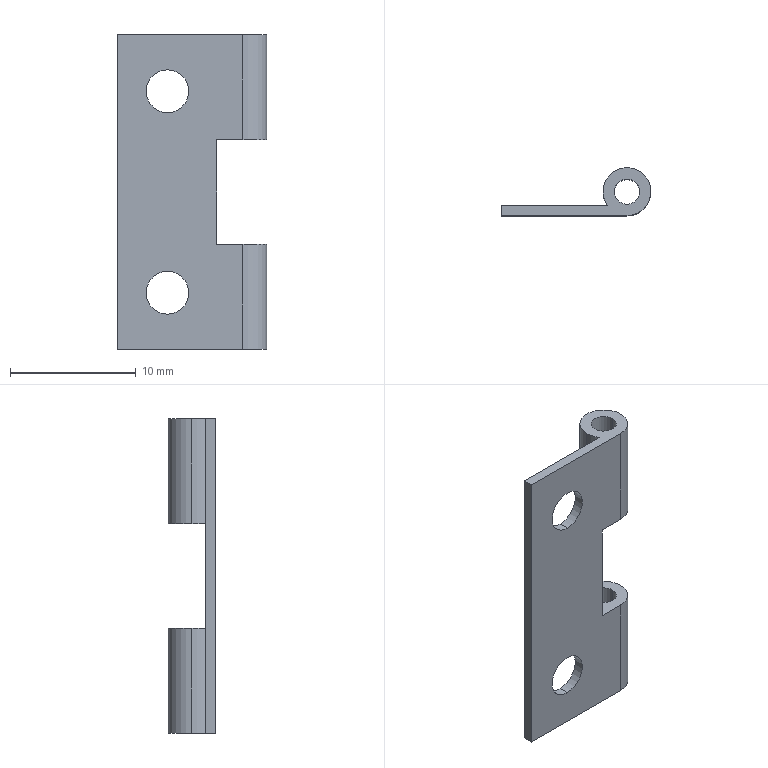Part | SolidWorks | features ICE 3, RefAxis 3, 3DProfileFeature 1, Extrusion 1 | 1 solid | 22 faces | box 11.9 x 3.8 x 25 mm | volume 293.72 mm3 | cylinder 14 | plane 8 | commonest cylinder face diameters 3.8 x6 2 x4 3.4 x4
STEP:
#1=CARTESIAN_POINT('',(-6.,0.8,-6.2));
#2=VERTEX_POINT('',#1);
#3=CARTESIAN_POINT('',(-6.,0.8,-2.8));
#4=VERTEX_POINT('',#3);
#5=CARTESIAN_POINT('',(-6.,0.8,-4.5));
#6=DIRECTION('',(0.,1.,0.));
#7=DIRECTION('',(0.,0.,1.));
#8=AXIS2_PLACEMENT_3D('',#5,#6,#7);
#9=CIRCLE('',#8,1.7);
#10=EDGE_CURVE('',#2,#4,#9,.T.);
#11=ORIENTED_EDGE('',*,*,#10,.T.);
#12=CARTESIAN_POINT('',(-6.,0.,-2.8));
#13=VERTEX_POINT('',#12);
#14=CARTESIAN_POINT('',(-6.,0.8,-2.8));
#15=DIRECTION('',(0.,-1.,0.));
#16=VECTOR('',#15,1000.);
#17=LINE('',#14,#16);
#18=EDGE_CURVE('',#4,#13,#17,.T.);
#19=ORIENTED_EDGE('',*,*,#18,.T.);
#20=CARTESIAN_POINT('',(-6.,0.,-6.2));
#21=VERTEX_POINT('',#20);
#22=CARTESIAN_POINT('',(-6.,0.,-4.5));
#23=DIRECTION('',(0.,1.,0.));
#24=DIRECTION('',(0.,0.,1.));
#25=AXIS2_PLACEMENT_3D('',#22,#23,#24);
#26=CIRCLE('',#25,1.7);
#27=EDGE_CURVE('',#21,#13,#26,.T.);
#28=ORIENTED_EDGE('',*,*,#27,.F.);
#29=CARTESIAN_POINT('',(-6.,0.8,-6.2));
#30=DIRECTION('',(0.,-1.,0.));
#31=VECTOR('',#30,1000.);
#32=LINE('',#29,#31);
#33=EDGE_CURVE('',#2,#21,#32,.T.);
#34=ORIENTED_EDGE('',*,*,#33,.F.);
#35=EDGE_LOOP('',(#11,#19,#28,#34));
#36=FACE_OUTER_BOUND('',#35,.T.);
#37=CARTESIAN_POINT('',(-6.,0.8,-4.5));
#38=DIRECTION('',(0.,-1.,0.));
#39=DIRECTION('',(0.,0.,-1.));
#40=AXIS2_PLACEMENT_3D('',#37,#38,#39);
#41=CYLINDRICAL_SURFACE('',#40,1.7);
#42=ADVANCED_FACE('',(#36),#41,.F.);
#43=CARTESIAN_POINT('',(-6.,0.8,-22.2));
#44=VERTEX_POINT('',#43);
#45=CARTESIAN_POINT('',(-6.,0.8,-18.8));
#46=VERTEX_POINT('',#45);
#47=CARTESIAN_POINT('',(-6.,0.8,-20.5));
#48=DIRECTION('',(0.,1.,0.));
#49=DIRECTION('',(0.,0.,1.));
#50=AXIS2_PLACEMENT_3D('',#47,#48,#49);
#51=CIRCLE('',#50,1.7);
#52=EDGE_CURVE('',#44,#46,#51,.T.);
#53=ORIENTED_EDGE('',*,*,#52,.T.);
#54=CARTESIAN_POINT('',(-6.,0.,-18.8));
#55=VERTEX_POINT('',#54);
#56=CARTESIAN_POINT('',(-6.,0.8,-18.8));
#57=DIRECTION('',(0.,-1.,0.));
#58=VECTOR('',#57,1000.);
#59=LINE('',#56,#58);
#60=EDGE_CURVE('',#46,#55,#59,.T.);
#61=ORIENTED_EDGE('',*,*,#60,.T.);
#62=CARTESIAN_POINT('',(-6.,0.,-22.2));
#63=VERTEX_POINT('',#62);
#64=CARTESIAN_POINT('',(-6.,0.,-20.5));
#65=DIRECTION('',(0.,1.,0.));
#66=DIRECTION('',(0.,0.,1.));
#67=AXIS2_PLACEMENT_3D('',#64,#65,#66);
#68=CIRCLE('',#67,1.7);
#69=EDGE_CURVE('',#63,#55,#68,.T.);
#70=ORIENTED_EDGE('',*,*,#69,.F.);
#71=CARTESIAN_POINT('',(-6.,0.8,-22.2));
#72=DIRECTION('',(0.,-1.,0.));
#73=VECTOR('',#72,1000.);
#74=LINE('',#71,#73);
#75=EDGE_CURVE('',#44,#63,#74,.T.);
#76=ORIENTED_EDGE('',*,*,#75,.F.);
#77=EDGE_LOOP('',(#53,#61,#70,#76));
#78=FACE_OUTER_BOUND('',#77,.T.);
#79=CARTESIAN_POINT('',(-6.,0.8,-20.5));
#80=DIRECTION('',(0.,-1.,0.));
#81=DIRECTION('',(0.,0.,-1.));
#82=AXIS2_PLACEMENT_3D('',#79,#80,#81);
#83=CYLINDRICAL_SURFACE('',#82,1.7);
#84=ADVANCED_FACE('',(#78),#83,.F.);
#85=CARTESIAN_POINT('',(-1.,1.9,-25.));
#86=VERTEX_POINT('',#85);
#87=CARTESIAN_POINT('',(1.,1.9,-25.));
#88=VERTEX_POINT('',#87);
#89=CARTESIAN_POINT('',(0.,1.9,-25.));
#90=DIRECTION('',(0.,0.,1.));
#91=DIRECTION('',(1.,0.,0.));
#92=AXIS2_PLACEMENT_3D('',#89,#90,#91);
#93=CIRCLE('',#92,1.);
#94=EDGE_CURVE('',#86,#88,#93,.T.);
#95=ORIENTED_EDGE('',*,*,#94,.F.);
#96=CARTESIAN_POINT('',(-1.,1.9,-16.667));
#97=VERTEX_POINT('',#96);
#98=CARTESIAN_POINT('',(-1.,1.9,-25.));
#99=DIRECTION('',(0.,0.,1.));
#100=VECTOR('',#99,1000.);
#101=LINE('',#98,#100);
#102=EDGE_CURVE('',#86,#97,#101,.T.);
#103=ORIENTED_EDGE('',*,*,#102,.T.);
#104=CARTESIAN_POINT('',(1.,1.9,-16.667));
#105=VERTEX_POINT('',#104);
#106=CARTESIAN_POINT('',(0.,1.9,-16.667));
#107=DIRECTION('',(0.,0.,-1.));
#108=DIRECTION('',(1.,0.,0.));
#109=AXIS2_PLACEMENT_3D('',#106,#107,#108);
#110=CIRCLE('',#109,1.);
#111=EDGE_CURVE('',#105,#97,#110,.T.);
#112=ORIENTED_EDGE('',*,*,#111,.F.);
#113=CARTESIAN_POINT('',(1.,1.9,-25.));
#114=DIRECTION('',(0.,0.,1.));
#115=VECTOR('',#114,1000.);
#116=LINE('',#113,#115);
#117=EDGE_CURVE('',#88,#105,#116,.T.);
#118=ORIENTED_EDGE('',*,*,#117,.F.);
#119=EDGE_LOOP('',(#95,#103,#112,#118));
#120=FACE_OUTER_BOUND('',#119,.T.);
#121=CARTESIAN_POINT('',(0.,1.9,-25.));
#122=DIRECTION('',(0.,0.,1.));
#123=DIRECTION('',(1.,0.,0.));
#124=AXIS2_PLACEMENT_3D('',#121,#122,#123);
#125=CYLINDRICAL_SURFACE('',#124,1.);
#126=ADVANCED_FACE('',(#120),#125,.F.);
#127=CARTESIAN_POINT('',(-1.,1.9,-8.333));
#128=VERTEX_POINT('',#127);
#129=CARTESIAN_POINT('',(1.,1.9,-8.333));
#130=VERTEX_POINT('',#129);
#131=CARTESIAN_POINT('',(0.,1.9,-8.333));
#132=DIRECTION('',(0.,0.,1.));
#133=DIRECTION('',(-1.,0.,0.));
#134=AXIS2_PLACEMENT_3D('',#131,#132,#133);
#135=CIRCLE('',#134,1.);
#136=EDGE_CURVE('',#128,#130,#135,.T.);
#137=ORIENTED_EDGE('',*,*,#136,.F.);
#138=CARTESIAN_POINT('',(-1.,1.9,0.));
#139=VERTEX_POINT('',#138);
#140=CARTESIAN_POINT('',(-1.,1.9,-25.));
#141=DIRECTION('',(0.,0.,1.));
#142=VECTOR('',#141,1000.);
#143=LINE('',#140,#142);
#144=EDGE_CURVE('',#128,#139,#143,.T.);
#145=ORIENTED_EDGE('',*,*,#144,.T.);
#146=CARTESIAN_POINT('',(1.,1.9,0.));
#147=VERTEX_POINT('',#146);
#148=CARTESIAN_POINT('',(0.,1.9,0.));
#149=DIRECTION('',(0.,0.,1.));
#150=DIRECTION('',(1.,0.,0.));
#151=AXIS2_PLACEMENT_3D('',#148,#149,#150);
#152=CIRCLE('',#151,1.);
#153=EDGE_CURVE('',#139,#147,#152,.T.);
#154=ORIENTED_EDGE('',*,*,#153,.T.);
#155=CARTESIAN_POINT('',(1.,1.9,-25.));
#156=DIRECTION('',(0.,0.,1.));
#157=VECTOR('',#156,1000.);
#158=LINE('',#155,#157);
#159=EDGE_CURVE('',#130,#147,#158,.T.);
#160=ORIENTED_EDGE('',*,*,#159,.F.);
#161=EDGE_LOOP('',(#137,#145,#154,#160));
#162=FACE_OUTER_BOUND('',#161,.T.);
#163=CARTESIAN_POINT('',(0.,1.9,-25.));
#164=DIRECTION('',(0.,0.,1.));
#165=DIRECTION('',(1.,0.,0.));
#166=AXIS2_PLACEMENT_3D('',#163,#164,#165);
#167=CYLINDRICAL_SURFACE('',#166,1.);
#168=ADVANCED_FACE('',(#162),#167,.F.);
#169=CARTESIAN_POINT('',(1.9,1.9,-25.));
#170=VERTEX_POINT('',#169);
#171=CARTESIAN_POINT('',(-1.9,1.9,-25.));
#172=VERTEX_POINT('',#171);
#173=CARTESIAN_POINT('',(0.,1.9,-25.));
#174=DIRECTION('',(0.,0.,1.));
#175=DIRECTION('',(1.,0.,0.));
#176=AXIS2_PLACEMENT_3D('',#173,#174,#175);
#177=CIRCLE('',#176,1.9);
#178=EDGE_CURVE('',#170,#172,#177,.T.);
#179=ORIENTED_EDGE('',*,*,#178,.T.);
#180=CARTESIAN_POINT('',(-1.9,1.9,-16.667));
#181=VERTEX_POINT('',#180);
#182=CARTESIAN_POINT('',(-1.9,1.9,-25.));
#183=DIRECTION('',(0.,0.,1.));
#184=VECTOR('',#183,1000.);
#185=LINE('',#182,#184);
#186=EDGE_CURVE('',#172,#181,#185,.T.);
#187=ORIENTED_EDGE('',*,*,#186,.T.);
#188=CARTESIAN_POINT('',(1.9,1.9,-16.667));
#189=VERTEX_POINT('',#188);
#190=CARTESIAN_POINT('',(0.,1.9,-16.667));
#191=DIRECTION('',(0.,0.,-1.));
#192=DIRECTION('',(1.,0.,0.));
#193=AXIS2_PLACEMENT_3D('',#190,#191,#192);
#194=CIRCLE('',#193,1.9);
#195=EDGE_CURVE('',#181,#189,#194,.T.);
#196=ORIENTED_EDGE('',*,*,#195,.T.);
#197=CARTESIAN_POINT('',(1.9,1.9,-25.));
#198=DIRECTION('',(0.,0.,1.));
#199=VECTOR('',#198,1000.);
#200=LINE('',#197,#199);
#201=EDGE_CURVE('',#170,#189,#200,.T.);
#202=ORIENTED_EDGE('',*,*,#201,.F.);
#203=EDGE_LOOP('',(#179,#187,#196,#202));
#204=FACE_OUTER_BOUND('',#203,.T.);
#205=CARTESIAN_POINT('',(0.,1.9,-25.));
#206=DIRECTION('',(0.,0.,1.));
#207=DIRECTION('',(1.,0.,0.));
#208=AXIS2_PLACEMENT_3D('',#205,#206,#207);
#209=CYLINDRICAL_SURFACE('',#208,1.9);
#210=ADVANCED_FACE('',(#204),#209,.T.);
#211=CARTESIAN_POINT('',(0.,0.,-25.));
#212=VERTEX_POINT('',#211);
#213=CARTESIAN_POINT('',(0.,1.9,-25.));
#214=DIRECTION('',(0.,0.,1.));
#215=DIRECTION('',(1.,0.,0.));
#216=AXIS2_PLACEMENT_3D('',#213,#214,#215);
#217=CIRCLE('',#216,1.9);
#218=EDGE_CURVE('',#212,#170,#217,.T.);
#219=ORIENTED_EDGE('',*,*,#218,.T.);
#220=ORIENTED_EDGE('',*,*,#201,.T.);
#221=CARTESIAN_POINT('',(0.,0.,-16.667));
#222=VERTEX_POINT('',#221);
#223=CARTESIAN_POINT('',(0.,1.9,-16.667));
#224=DIRECTION('',(0.,0.,-1.));
#225=DIRECTION('',(1.,0.,0.));
#226=AXIS2_PLACEMENT_3D('',#223,#224,#225);
#227=CIRCLE('',#226,1.9);
#228=EDGE_CURVE('',#189,#222,#227,.T.);
#229=ORIENTED_EDGE('',*,*,#228,.T.);
#230=CARTESIAN_POINT('',(0.,0.,-25.));
#231=DIRECTION('',(0.,0.,1.));
#232=VECTOR('',#231,1000.);
#233=LINE('',#230,#232);
#234=EDGE_CURVE('',#212,#222,#233,.T.);
#235=ORIENTED_EDGE('',*,*,#234,.F.);
#236=EDGE_LOOP('',(#219,#220,#229,#235));
#237=FACE_OUTER_BOUND('',#236,.T.);
#238=CARTESIAN_POINT('',(0.,1.9,-25.));
#239=DIRECTION('',(0.,0.,1.));
#240=DIRECTION('',(1.,0.,0.));
#241=AXIS2_PLACEMENT_3D('',#238,#239,#240);
#242=CYLINDRICAL_SURFACE('',#241,1.9);
#243=ADVANCED_FACE('',(#237),#242,.T.);
#244=CARTESIAN_POINT('',(1.9,1.9,-8.333));
#245=VERTEX_POINT('',#244);
#246=CARTESIAN_POINT('',(-1.9,1.9,-8.333));
#247=VERTEX_POINT('',#246);
#248=CARTESIAN_POINT('',(0.,1.9,-8.333));
#249=DIRECTION('',(0.,0.,1.));
#250=DIRECTION('',(-1.,0.,0.));
#251=AXIS2_PLACEMENT_3D('',#248,#249,#250);
#252=CIRCLE('',#251,1.9);
#253=EDGE_CURVE('',#245,#247,#252,.T.);
#254=ORIENTED_EDGE('',*,*,#253,.T.);
#255=CARTESIAN_POINT('',(-1.9,1.9,0.));
#256=VERTEX_POINT('',#255);
#257=CARTESIAN_POINT('',(-1.9,1.9,-25.));
#258=DIRECTION('',(0.,0.,1.));
#259=VECTOR('',#258,1000.);
#260=LINE('',#257,#259);
#261=EDGE_CURVE('',#247,#256,#260,.T.);
#262=ORIENTED_EDGE('',*,*,#261,.T.);
#263=CARTESIAN_POINT('',(1.9,1.9,0.));
#264=VERTEX_POINT('',#263);
#265=CARTESIAN_POINT('',(0.,1.9,0.));
#266=DIRECTION('',(0.,0.,1.));
#267=DIRECTION('',(1.,0.,0.));
#268=AXIS2_PLACEMENT_3D('',#265,#266,#267);
#269=CIRCLE('',#268,1.9);
#270=EDGE_CURVE('',#264,#256,#269,.T.);
#271=ORIENTED_EDGE('',*,*,#270,.F.);
#272=CARTESIAN_POINT('',(1.9,1.9,-25.));
#273=DIRECTION('',(0.,0.,1.));
#274=VECTOR('',#273,1000.);
#275=LINE('',#272,#274);
#276=EDGE_CURVE('',#245,#264,#275,.T.);
#277=ORIENTED_EDGE('',*,*,#276,.F.);
#278=EDGE_LOOP('',(#254,#262,#271,#277));
#279=FACE_OUTER_BOUND('',#278,.T.);
#280=CARTESIAN_POINT('',(0.,1.9,-25.));
#281=DIRECTION('',(0.,0.,1.));
#282=DIRECTION('',(1.,0.,0.));
#283=AXIS2_PLACEMENT_3D('',#280,#281,#282);
#284=CYLINDRICAL_SURFACE('',#283,1.9);
#285=ADVANCED_FACE('',(#279),#284,.T.);
#286=CARTESIAN_POINT('',(0.,0.,-8.333));
#287=VERTEX_POINT('',#286);
#288=CARTESIAN_POINT('',(0.,1.9,-8.333));
#289=DIRECTION('',(0.,0.,1.));
#290=DIRECTION('',(-1.,0.,0.));
#291=AXIS2_PLACEMENT_3D('',#288,#289,#290);
#292=CIRCLE('',#291,1.9);
#293=EDGE_CURVE('',#287,#245,#292,.T.);
#294=ORIENTED_EDGE('',*,*,#293,.T.);
#295=ORIENTED_EDGE('',*,*,#276,.T.);
#296=CARTESIAN_POINT('',(0.,0.,0.));
#297=VERTEX_POINT('',#296);
#298=CARTESIAN_POINT('',(0.,1.9,0.));
#299=DIRECTION('',(0.,0.,1.));
#300=DIRECTION('',(1.,0.,0.));
#301=AXIS2_PLACEMENT_3D('',#298,#299,#300);
#302=CIRCLE('',#301,1.9);
#303=EDGE_CURVE('',#297,#264,#302,.T.);
#304=ORIENTED_EDGE('',*,*,#303,.F.);
#305=CARTESIAN_POINT('',(0.,0.,-25.));
#306=DIRECTION('',(0.,0.,1.));
#307=VECTOR('',#306,1000.);
#308=LINE('',#305,#307);
#309=EDGE_CURVE('',#287,#297,#308,.T.);
#310=ORIENTED_EDGE('',*,*,#309,.F.);
#311=EDGE_LOOP('',(#294,#295,#304,#310));
#312=FACE_OUTER_BOUND('',#311,.T.);
#313=CARTESIAN_POINT('',(0.,1.9,-25.));
#314=DIRECTION('',(0.,0.,1.));
#315=DIRECTION('',(1.,0.,0.));
#316=AXIS2_PLACEMENT_3D('',#313,#314,#315);
#317=CYLINDRICAL_SURFACE('',#316,1.9);
#318=ADVANCED_FACE('',(#312),#317,.T.);
#319=ORIENTED_EDGE('',*,*,#52,.F.);
#320=CARTESIAN_POINT('',(-6.,0.8,-20.5));
#321=DIRECTION('',(0.,1.,0.));
#322=DIRECTION('',(0.,0.,1.));
#323=AXIS2_PLACEMENT_3D('',#320,#321,#322);
#324=CIRCLE('',#323,1.7);
#325=EDGE_CURVE('',#46,#44,#324,.T.);
#326=ORIENTED_EDGE('',*,*,#325,.F.);
#327=EDGE_LOOP('',(#319,#326));
#328=FACE_BOUND('',#327,.T.);
#329=CARTESIAN_POINT('',(-1.549,0.8,-8.333));
#330=VERTEX_POINT('',#329);
#331=CARTESIAN_POINT('',(-1.549,0.8,0.));
#332=VERTEX_POINT('',#331);
#333=CARTESIAN_POINT('',(-1.549,0.8,-25.));
#334=DIRECTION('',(0.,0.,1.));
#335=VECTOR('',#334,1000.);
#336=LINE('',#333,#335);
#337=EDGE_CURVE('',#330,#332,#336,.T.);
#338=ORIENTED_EDGE('',*,*,#337,.F.);
#339=CARTESIAN_POINT('',(-2.09,0.8,-8.333));
#340=VERTEX_POINT('',#339);
#341=CARTESIAN_POINT('',(-1.549,0.8,-8.333));
#342=DIRECTION('',(-1.,0.,0.));
#343=VECTOR('',#342,1000.);
#344=LINE('',#341,#343);
#345=EDGE_CURVE('',#330,#340,#344,.T.);
#346=ORIENTED_EDGE('',*,*,#345,.T.);
#347=CARTESIAN_POINT('',(-2.09,0.8,-16.667));
#348=VERTEX_POINT('',#347);
#349=CARTESIAN_POINT('',(-2.09,0.8,-25.));
#350=DIRECTION('',(0.,0.,-1.));
#351=VECTOR('',#350,1000.);
#352=LINE('',#349,#351);
#353=EDGE_CURVE('',#340,#348,#352,.T.);
#354=ORIENTED_EDGE('',*,*,#353,.T.);
#355=CARTESIAN_POINT('',(-1.549,0.8,-16.667));
#356=VERTEX_POINT('',#355);
#357=CARTESIAN_POINT('',(-1.549,0.8,-16.667));
#358=DIRECTION('',(1.,0.,0.));
#359=VECTOR('',#358,1000.);
#360=LINE('',#357,#359);
#361=EDGE_CURVE('',#348,#356,#360,.T.);
#362=ORIENTED_EDGE('',*,*,#361,.T.);
#363=CARTESIAN_POINT('',(-1.549,0.8,-25.));
#364=VERTEX_POINT('',#363);
#365=CARTESIAN_POINT('',(-1.549,0.8,-25.));
#366=DIRECTION('',(0.,0.,1.));
#367=VECTOR('',#366,1000.);
#368=LINE('',#365,#367);
#369=EDGE_CURVE('',#364,#356,#368,.T.);
#370=ORIENTED_EDGE('',*,*,#369,.F.);
#371=CARTESIAN_POINT('',(-10.,0.8,-25.));
#372=VERTEX_POINT('',#371);
#373=CARTESIAN_POINT('',(-1.549,0.8,-25.));
#374=DIRECTION('',(-1.,0.,0.));
#375=VECTOR('',#374,1000.);
#376=LINE('',#373,#375);
#377=EDGE_CURVE('',#364,#372,#376,.T.);
#378=ORIENTED_EDGE('',*,*,#377,.T.);
#379=CARTESIAN_POINT('',(-10.,0.8,0.));
#380=VERTEX_POINT('',#379);
#381=CARTESIAN_POINT('',(-10.,0.8,-25.));
#382=DIRECTION('',(0.,0.,1.));
#383=VECTOR('',#382,1000.);
#384=LINE('',#381,#383);
#385=EDGE_CURVE('',#372,#380,#384,.T.);
#386=ORIENTED_EDGE('',*,*,#385,.T.);
#387=CARTESIAN_POINT('',(-1.549,0.8,0.));
#388=DIRECTION('',(-1.,0.,0.));
#389=VECTOR('',#388,1000.);
#390=LINE('',#387,#389);
#391=EDGE_CURVE('',#332,#380,#390,.T.);
#392=ORIENTED_EDGE('',*,*,#391,.F.);
#393=EDGE_LOOP('',(#338,#346,#354,#362,#370,#378,#386,#392));
#394=FACE_OUTER_BOUND('',#393,.T.);
#395=ORIENTED_EDGE('',*,*,#10,.F.);
#396=CARTESIAN_POINT('',(-6.,0.8,-4.5));
#397=DIRECTION('',(0.,1.,0.));
#398=DIRECTION('',(0.,0.,1.));
#399=AXIS2_PLACEMENT_3D('',#396,#397,#398);
#400=CIRCLE('',#399,1.7);
#401=EDGE_CURVE('',#4,#2,#400,.T.);
#402=ORIENTED_EDGE('',*,*,#401,.F.);
#403=EDGE_LOOP('',(#395,#402));
#404=FACE_BOUND('',#403,.T.);
#405=CARTESIAN_POINT('',(-1.549,0.8,-25.));
#406=DIRECTION('',(0.,1.,0.));
#407=DIRECTION('',(0.,0.,1.));
#408=AXIS2_PLACEMENT_3D('',#405,#406,#407);
#409=PLANE('',#408);
#410=ADVANCED_FACE('',(#328,#394,#404),#409,.T.);
#411=ORIENTED_EDGE('',*,*,#69,.T.);
#412=CARTESIAN_POINT('',(-6.,0.,-20.5));
#413=DIRECTION('',(0.,1.,0.));
#414=DIRECTION('',(0.,0.,1.));
#415=AXIS2_PLACEMENT_3D('',#412,#413,#414);
#416=CIRCLE('',#415,1.7);
#417=EDGE_CURVE('',#55,#63,#416,.T.);
#418=ORIENTED_EDGE('',*,*,#417,.T.);
#419=EDGE_LOOP('',(#411,#418));
#420=FACE_BOUND('',#419,.T.);
#421=CARTESIAN_POINT('',(-2.09,0.,-16.667));
#422=VERTEX_POINT('',#421);
#423=CARTESIAN_POINT('',(-2.09,0.,-8.333));
#424=VERTEX_POINT('',#423);
#425=CARTESIAN_POINT('',(-2.09,0.,-16.667));
#426=DIRECTION('',(0.,0.,1.));
#427=VECTOR('',#426,1000.);
#428=LINE('',#425,#427);
#429=EDGE_CURVE('',#422,#424,#428,.T.);
#430=ORIENTED_EDGE('',*,*,#429,.T.);
#431=CARTESIAN_POINT('',(-2.09,0.,-8.333));
#432=DIRECTION('',(1.,0.,0.));
#433=VECTOR('',#432,1000.);
#434=LINE('',#431,#433);
#435=EDGE_CURVE('',#424,#287,#434,.T.);
#436=ORIENTED_EDGE('',*,*,#435,.T.);
#437=ORIENTED_EDGE('',*,*,#309,.T.);
#438=CARTESIAN_POINT('',(-10.,0.,0.));
#439=VERTEX_POINT('',#438);
#440=CARTESIAN_POINT('',(-10.,0.,0.));
#441=DIRECTION('',(1.,0.,0.));
#442=VECTOR('',#441,1000.);
#443=LINE('',#440,#442);
#444=EDGE_CURVE('',#439,#297,#443,.T.);
#445=ORIENTED_EDGE('',*,*,#444,.F.);
#446=CARTESIAN_POINT('',(-10.,0.,-25.));
#447=VERTEX_POINT('',#446);
#448=CARTESIAN_POINT('',(-10.,0.,-25.));
#449=DIRECTION('',(0.,0.,1.));
#450=VECTOR('',#449,1000.);
#451=LINE('',#448,#450);
#452=EDGE_CURVE('',#447,#439,#451,.T.);
#453=ORIENTED_EDGE('',*,*,#452,.F.);
#454=CARTESIAN_POINT('',(-10.,0.,-25.));
#455=DIRECTION('',(1.,0.,0.));
#456=VECTOR('',#455,1000.);
#457=LINE('',#454,#456);
#458=EDGE_CURVE('',#447,#212,#457,.T.);
#459=ORIENTED_EDGE('',*,*,#458,.T.);
#460=ORIENTED_EDGE('',*,*,#234,.T.);
#461=CARTESIAN_POINT('',(2.09,0.,-16.667));
#462=DIRECTION('',(-1.,0.,0.));
#463=VECTOR('',#462,1000.);
#464=LINE('',#461,#463);
#465=EDGE_CURVE('',#222,#422,#464,.T.);
#466=ORIENTED_EDGE('',*,*,#465,.T.);
#467=EDGE_LOOP('',(#430,#436,#437,#445,#453,#459,#460,#466));
#468=FACE_OUTER_BOUND('',#467,.T.);
#469=ORIENTED_EDGE('',*,*,#27,.T.);
#470=CARTESIAN_POINT('',(-6.,0.,-4.5));
#471=DIRECTION('',(0.,1.,0.));
#472=DIRECTION('',(0.,0.,1.));
#473=AXIS2_PLACEMENT_3D('',#470,#471,#472);
#474=CIRCLE('',#473,1.7);
#475=EDGE_CURVE('',#13,#21,#474,.T.);
#476=ORIENTED_EDGE('',*,*,#475,.T.);
#477=EDGE_LOOP('',(#469,#476));
#478=FACE_BOUND('',#477,.T.);
#479=CARTESIAN_POINT('',(-10.,0.,-25.));
#480=DIRECTION('',(0.,-1.,0.));
#481=DIRECTION('',(0.,0.,-1.));
#482=AXIS2_PLACEMENT_3D('',#479,#480,#481);
#483=PLANE('',#482);
#484=ADVANCED_FACE('',(#420,#468,#478),#483,.T.);
#485=ORIENTED_EDGE('',*,*,#261,.F.);
#486=CARTESIAN_POINT('',(0.,1.9,-8.333));
#487=DIRECTION('',(0.,0.,1.));
#488=DIRECTION('',(-1.,0.,0.));
#489=AXIS2_PLACEMENT_3D('',#486,#487,#488);
#490=CIRCLE('',#489,1.9);
#491=EDGE_CURVE('',#247,#330,#490,.T.);
#492=ORIENTED_EDGE('',*,*,#491,.T.);
#493=ORIENTED_EDGE('',*,*,#337,.T.);
#494=CARTESIAN_POINT('',(0.,1.9,0.));
#495=DIRECTION('',(0.,0.,1.));
#496=DIRECTION('',(1.,0.,0.));
#497=AXIS2_PLACEMENT_3D('',#494,#495,#496);
#498=CIRCLE('',#497,1.9);
#499=EDGE_CURVE('',#256,#332,#498,.T.);
#500=ORIENTED_EDGE('',*,*,#499,.F.);
#501=EDGE_LOOP('',(#485,#492,#493,#500));
#502=FACE_OUTER_BOUND('',#501,.T.);
#503=CARTESIAN_POINT('',(0.,1.9,-25.));
#504=DIRECTION('',(0.,0.,1.));
#505=DIRECTION('',(1.,0.,0.));
#506=AXIS2_PLACEMENT_3D('',#503,#504,#505);
#507=CYLINDRICAL_SURFACE('',#506,1.9);
#508=ADVANCED_FACE('',(#502),#507,.T.);
#509=ORIENTED_EDGE('',*,*,#186,.F.);
#510=CARTESIAN_POINT('',(0.,1.9,-25.));
#511=DIRECTION('',(0.,0.,1.));
#512=DIRECTION('',(1.,0.,0.));
#513=AXIS2_PLACEMENT_3D('',#510,#511,#512);
#514=CIRCLE('',#513,1.9);
#515=EDGE_CURVE('',#172,#364,#514,.T.);
#516=ORIENTED_EDGE('',*,*,#515,.T.);
#517=ORIENTED_EDGE('',*,*,#369,.T.);
#518=CARTESIAN_POINT('',(0.,1.9,-16.667));
#519=DIRECTION('',(0.,0.,-1.));
#520=DIRECTION('',(1.,0.,0.));
#521=AXIS2_PLACEMENT_3D('',#518,#519,#520);
#522=CIRCLE('',#521,1.9);
#523=EDGE_CURVE('',#356,#181,#522,.T.);
#524=ORIENTED_EDGE('',*,*,#523,.T.);
#525=EDGE_LOOP('',(#509,#516,#517,#524));
#526=FACE_OUTER_BOUND('',#525,.T.);
#527=CARTESIAN_POINT('',(0.,1.9,-25.));
#528=DIRECTION('',(0.,0.,1.));
#529=DIRECTION('',(1.,0.,0.));
#530=AXIS2_PLACEMENT_3D('',#527,#528,#529);
#531=CYLINDRICAL_SURFACE('',#530,1.9);
#532=ADVANCED_FACE('',(#526),#531,.T.);
#533=ORIENTED_EDGE('',*,*,#144,.F.);
#534=CARTESIAN_POINT('',(0.,1.9,-8.333));
#535=DIRECTION('',(0.,0.,1.));
#536=DIRECTION('',(-1.,0.,0.));
#537=AXIS2_PLACEMENT_3D('',#534,#535,#536);
#538=CIRCLE('',#537,1.);
#539=EDGE_CURVE('',#130,#128,#538,.T.);
#540=ORIENTED_EDGE('',*,*,#539,.F.);
#541=ORIENTED_EDGE('',*,*,#159,.T.);
#542=CARTESIAN_POINT('',(0.,1.9,0.));
#543=DIRECTION('',(0.,0.,1.));
#544=DIRECTION('',(1.,0.,0.));
#545=AXIS2_PLACEMENT_3D('',#542,#543,#544);
#546=CIRCLE('',#545,1.);
#547=EDGE_CURVE('',#147,#139,#546,.T.);
#548=ORIENTED_EDGE('',*,*,#547,.T.);
#549=EDGE_LOOP('',(#533,#540,#541,#548));
#550=FACE_OUTER_BOUND('',#549,.T.);
#551=CARTESIAN_POINT('',(0.,1.9,-25.));
#552=DIRECTION('',(0.,0.,1.));
#553=DIRECTION('',(1.,0.,0.));
#554=AXIS2_PLACEMENT_3D('',#551,#552,#553);
#555=CYLINDRICAL_SURFACE('',#554,1.);
#556=ADVANCED_FACE('',(#550),#555,.F.);
#557=ORIENTED_EDGE('',*,*,#102,.F.);
#558=CARTESIAN_POINT('',(0.,1.9,-25.));
#559=DIRECTION('',(0.,0.,1.));
#560=DIRECTION('',(1.,0.,0.));
#561=AXIS2_PLACEMENT_3D('',#558,#559,#560);
#562=CIRCLE('',#561,1.);
#563=EDGE_CURVE('',#88,#86,#562,.T.);
#564=ORIENTED_EDGE('',*,*,#563,.F.);
#565=ORIENTED_EDGE('',*,*,#117,.T.);
#566=CARTESIAN_POINT('',(0.,1.9,-16.667));
#567=DIRECTION('',(0.,0.,-1.));
#568=DIRECTION('',(1.,0.,0.));
#569=AXIS2_PLACEMENT_3D('',#566,#567,#568);
#570=CIRCLE('',#569,1.);
#571=EDGE_CURVE('',#97,#105,#570,.T.);
#572=ORIENTED_EDGE('',*,*,#571,.F.);
#573=EDGE_LOOP('',(#557,#564,#565,#572));
#574=FACE_OUTER_BOUND('',#573,.T.);
#575=CARTESIAN_POINT('',(0.,1.9,-25.));
#576=DIRECTION('',(0.,0.,1.));
#577=DIRECTION('',(1.,0.,0.));
#578=AXIS2_PLACEMENT_3D('',#575,#576,#577);
#579=CYLINDRICAL_SURFACE('',#578,1.);
#580=ADVANCED_FACE('',(#574),#579,.F.);
#581=CARTESIAN_POINT('',(-10.,0.8,0.));
#582=DIRECTION('',(0.,-1.,0.));
#583=VECTOR('',#582,1000.);
#584=LINE('',#581,#583);
#585=EDGE_CURVE('',#380,#439,#584,.T.);
#586=ORIENTED_EDGE('',*,*,#585,.F.);
#587=ORIENTED_EDGE('',*,*,#385,.F.);
#588=CARTESIAN_POINT('',(-10.,0.8,-25.));
#589=DIRECTION('',(0.,-1.,0.));
#590=VECTOR('',#589,1000.);
#591=LINE('',#588,#590);
#592=EDGE_CURVE('',#372,#447,#591,.T.);
#593=ORIENTED_EDGE('',*,*,#592,.T.);
#594=ORIENTED_EDGE('',*,*,#452,.T.);
#595=EDGE_LOOP('',(#586,#587,#593,#594));
#596=FACE_OUTER_BOUND('',#595,.T.);
#597=CARTESIAN_POINT('',(-10.,0.8,-25.));
#598=DIRECTION('',(-1.,0.,0.));
#599=DIRECTION('',(0.,0.,1.));
#600=AXIS2_PLACEMENT_3D('',#597,#598,#599);
#601=PLANE('',#600);
#602=ADVANCED_FACE('',(#596),#601,.T.);
#603=ORIENTED_EDGE('',*,*,#563,.T.);
#604=ORIENTED_EDGE('',*,*,#94,.T.);
#605=EDGE_LOOP('',(#603,#604));
#606=FACE_BOUND('',#605,.T.);
#607=ORIENTED_EDGE('',*,*,#592,.F.);
#608=ORIENTED_EDGE('',*,*,#377,.F.);
#609=ORIENTED_EDGE('',*,*,#515,.F.);
#610=ORIENTED_EDGE('',*,*,#178,.F.);
#611=ORIENTED_EDGE('',*,*,#218,.F.);
#612=ORIENTED_EDGE('',*,*,#458,.F.);
#613=EDGE_LOOP('',(#607,#608,#609,#610,#611,#612));
#614=FACE_OUTER_BOUND('',#613,.T.);
#615=CARTESIAN_POINT('',(0.,1.9,-25.));
#616=DIRECTION('',(0.,0.,1.));
#617=DIRECTION('',(1.,0.,0.));
#618=AXIS2_PLACEMENT_3D('',#615,#616,#617);
#619=PLANE('',#618);
#620=ADVANCED_FACE('',(#606,#614),#619,.F.);
#621=ORIENTED_EDGE('',*,*,#547,.F.);
#622=ORIENTED_EDGE('',*,*,#153,.F.);
#623=EDGE_LOOP('',(#621,#622));
#624=FACE_BOUND('',#623,.T.);
#625=ORIENTED_EDGE('',*,*,#585,.T.);
#626=ORIENTED_EDGE('',*,*,#444,.T.);
#627=ORIENTED_EDGE('',*,*,#303,.T.);
#628=ORIENTED_EDGE('',*,*,#270,.T.);
#629=ORIENTED_EDGE('',*,*,#499,.T.);
#630=ORIENTED_EDGE('',*,*,#391,.T.);
#631=EDGE_LOOP('',(#625,#626,#627,#628,#629,#630));
#632=FACE_OUTER_BOUND('',#631,.T.);
#633=CARTESIAN_POINT('',(0.,1.9,0.));
#634=DIRECTION('',(0.,0.,1.));
#635=DIRECTION('',(1.,0.,0.));
#636=AXIS2_PLACEMENT_3D('',#633,#634,#635);
#637=PLANE('',#636);
#638=ADVANCED_FACE('',(#624,#632),#637,.T.);
#639=ORIENTED_EDGE('',*,*,#293,.F.);
#640=ORIENTED_EDGE('',*,*,#435,.F.);
#641=CARTESIAN_POINT('',(-2.09,3.8,-8.333));
#642=DIRECTION('',(0.,-1.,0.));
#643=VECTOR('',#642,1000.);
#644=LINE('',#641,#643);
#645=EDGE_CURVE('',#340,#424,#644,.T.);
#646=ORIENTED_EDGE('',*,*,#645,.F.);
#647=ORIENTED_EDGE('',*,*,#345,.F.);
#648=ORIENTED_EDGE('',*,*,#491,.F.);
#649=ORIENTED_EDGE('',*,*,#253,.F.);
#650=EDGE_LOOP('',(#639,#640,#646,#647,#648,#649));
#651=FACE_OUTER_BOUND('',#650,.T.);
#652=ORIENTED_EDGE('',*,*,#539,.T.);
#653=ORIENTED_EDGE('',*,*,#136,.T.);
#654=EDGE_LOOP('',(#652,#653));
#655=FACE_BOUND('',#654,.T.);
#656=CARTESIAN_POINT('',(-2.09,3.8,-8.333));
#657=DIRECTION('',(0.,0.,-1.));
#658=DIRECTION('',(-1.,0.,0.));
#659=AXIS2_PLACEMENT_3D('',#656,#657,#658);
#660=PLANE('',#659);
#661=ADVANCED_FACE('',(#651,#655),#660,.T.);
#662=CARTESIAN_POINT('',(-2.09,3.8,-16.667));
#663=DIRECTION('',(0.,-1.,0.));
#664=VECTOR('',#663,1000.);
#665=LINE('',#662,#664);
#666=EDGE_CURVE('',#348,#422,#665,.T.);
#667=ORIENTED_EDGE('',*,*,#666,.T.);
#668=ORIENTED_EDGE('',*,*,#465,.F.);
#669=ORIENTED_EDGE('',*,*,#228,.F.);
#670=ORIENTED_EDGE('',*,*,#195,.F.);
#671=ORIENTED_EDGE('',*,*,#523,.F.);
#672=ORIENTED_EDGE('',*,*,#361,.F.);
#673=EDGE_LOOP('',(#667,#668,#669,#670,#671,#672));
#674=FACE_OUTER_BOUND('',#673,.T.);
#675=ORIENTED_EDGE('',*,*,#111,.T.);
#676=ORIENTED_EDGE('',*,*,#571,.T.);
#677=EDGE_LOOP('',(#675,#676));
#678=FACE_BOUND('',#677,.T.);
#679=CARTESIAN_POINT('',(2.09,3.8,-16.667));
#680=DIRECTION('',(0.,0.,1.));
#681=DIRECTION('',(1.,0.,0.));
#682=AXIS2_PLACEMENT_3D('',#679,#680,#681);
#683=PLANE('',#682);
#684=ADVANCED_FACE('',(#674,#678),#683,.T.);
#685=ORIENTED_EDGE('',*,*,#645,.T.);
#686=ORIENTED_EDGE('',*,*,#429,.F.);
#687=ORIENTED_EDGE('',*,*,#666,.F.);
#688=ORIENTED_EDGE('',*,*,#353,.F.);
#689=EDGE_LOOP('',(#685,#686,#687,#688));
#690=FACE_OUTER_BOUND('',#689,.T.);
#691=CARTESIAN_POINT('',(-2.09,3.8,-16.667));
#692=DIRECTION('',(1.,0.,0.));
#693=DIRECTION('',(0.,0.,-1.));
#694=AXIS2_PLACEMENT_3D('',#691,#692,#693);
#695=PLANE('',#694);
#696=ADVANCED_FACE('',(#690),#695,.T.);
#697=ORIENTED_EDGE('',*,*,#60,.F.);
#698=ORIENTED_EDGE('',*,*,#325,.T.);
#699=ORIENTED_EDGE('',*,*,#75,.T.);
#700=ORIENTED_EDGE('',*,*,#417,.F.);
#701=EDGE_LOOP('',(#697,#698,#699,#700));
#702=FACE_OUTER_BOUND('',#701,.T.);
#703=CARTESIAN_POINT('',(-6.,0.8,-20.5));
#704=DIRECTION('',(0.,-1.,0.));
#705=DIRECTION('',(0.,0.,-1.));
#706=AXIS2_PLACEMENT_3D('',#703,#704,#705);
#707=CYLINDRICAL_SURFACE('',#706,1.7);
#708=ADVANCED_FACE('',(#702),#707,.F.);
#709=ORIENTED_EDGE('',*,*,#18,.F.);
#710=ORIENTED_EDGE('',*,*,#401,.T.);
#711=ORIENTED_EDGE('',*,*,#33,.T.);
#712=ORIENTED_EDGE('',*,*,#475,.F.);
#713=EDGE_LOOP('',(#709,#710,#711,#712));
#714=FACE_OUTER_BOUND('',#713,.T.);
#715=CARTESIAN_POINT('',(-6.,0.8,-4.5));
#716=DIRECTION('',(0.,-1.,0.));
#717=DIRECTION('',(0.,0.,-1.));
#718=AXIS2_PLACEMENT_3D('',#715,#716,#717);
#719=CYLINDRICAL_SURFACE('',#718,1.7);
#720=ADVANCED_FACE('',(#714),#719,.F.);
#721=CLOSED_SHELL('',(#42,#84,#126,#168,#210,#243,#285,#318,#410,#484,#508,#532,#556,#580,#602,#620,#638,#661,#684,#696,#708,#720));
#722=MANIFOLD_SOLID_BREP('',#721);
#723=CARTESIAN_POINT('',(0.,0.,0.));
#724=DIRECTION('',(0.,0.,1.));
#725=DIRECTION('',(1.,0.,0.));
#726=AXIS2_PLACEMENT_3D('',#723,#724,#725);
#727=(LENGTH_UNIT()NAMED_UNIT(*)SI_UNIT(.MILLI.,.METRE.));
#728=UNCERTAINTY_MEASURE_WITH_UNIT(LENGTH_MEASURE(0.00001),#727,'','');
#729=(NAMED_UNIT(*)PLANE_ANGLE_UNIT()SI_UNIT($,.RADIAN.));
#730=(NAMED_UNIT(*)SI_UNIT($,.STERADIAN.)SOLID_ANGLE_UNIT());
#731=(GEOMETRIC_REPRESENTATION_CONTEXT(3)GLOBAL_UNCERTAINTY_ASSIGNED_CONTEXT((#728))GLOBAL_UNIT_ASSIGNED_CONTEXT((#727,#729,#730))REPRESENTATION_CONTEXT('',''));
#732=ADVANCED_BREP_SHAPE_REPRESENTATION('',(#722,#726),#731);